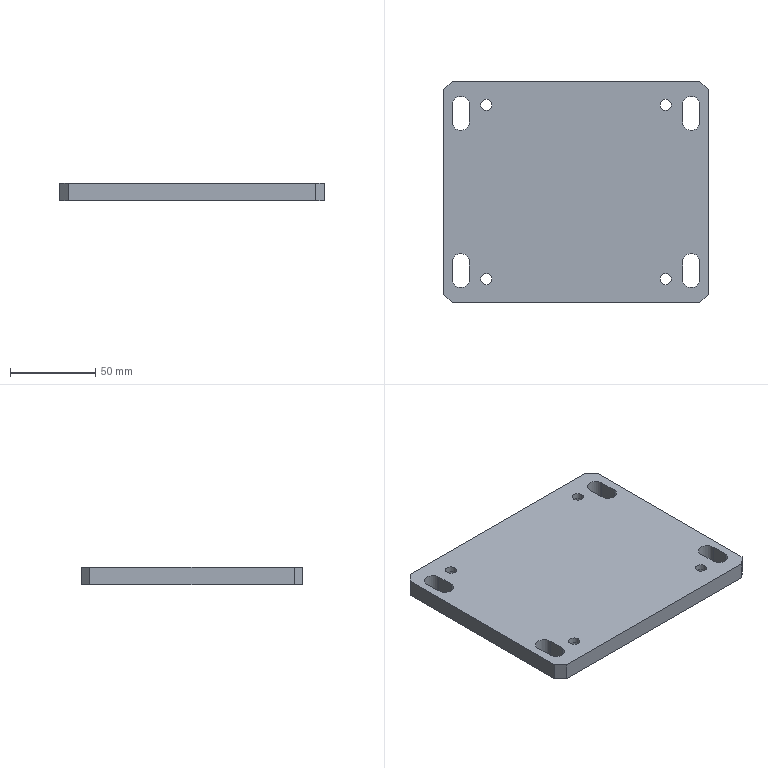CAM job | NX | 3-axis milling, drilling | part box 155 x 130 x 10 mm | stock box 155 x 130 x 10 mm
Tools:
number,name,description,diameter,corner_radius,flute_length,length,flutes
6,D6,平底铣刀-粗,6.0,0.0,25.0,75.0,2
9,D10,平底铣刀-粗,10.0,0.0,35.0,75.0,2
7,D6-J,平底铣刀-精,6.0,0.0,25.0,75.0,2
10,D10-J,平底铣刀-精,10.0,0.0,35.0,75.0,2
2,D6倒角刀,倒角刀,6.0,0.0,3.0,25.0,2
1,C6定点钻,倒角刀,6.0,0.0,3.0,3.0,2
17,ZT6.5,钻头,6.5,0.0,35.0,50.0,2
Operations:
program,operation,operation_type,tool,method,geometry_group,spindle_rpm,surface_speed,feed_per_tooth,feed_cut,feed_plunge,cut_length_mm,path_length_mm,cut_time_min,machine_time_min
B,选线往复层切开粗-中_COPY_1,PlanarMilling,D10,分层开粗-切深K-步距G,W-B,3000.0,94.245,0.3333,2000.0,100.0,1805.117,2433.317,0.9026,0.9654
B,铣倒角_2,PlanarMilling,D6倒角刀,METHOD,W-B,4000.0,75.398,0.075,600.0,100.0,76.787,554.602,0.128,0.1758
B,平面去毛刺6X45L_COPY_1,SurfaceContour,D6倒角刀,爬面_倒角-切深0-步距G,W-B,3500.0,65.972,0.1429,1000.0,100.0,835.116,1413.241,0.8351,0.8929
B,平面铣精光侧面-中-直线_COPY_1,PlanarMilling,D10-J,侧刃精光-切深K-步距G,W-B,3000.0,94.245,0.1333,800.0,100.0,84.284,661.042,0.1054,0.163
A,选线往复层切开粗-中_COPY,PlanarMilling,D10,分层开粗-切深K-步距G,W-A,3000.0,94.245,0.3333,2000.0,100.0,1805.117,2433.317,0.9026,0.9654
A,沉头孔打点-深0.8,Operation,C6定点钻,NONE,W-A,3000.0,56.0,0.01,60.0,90.0,7.2,366.415,0.12,0.1559
A,沉头孔-钻孔0段,Operation,ZT6.5,NONE,W-A,600.0,12.252,0.1,120.0,90.0,59.811,471.637,0.4984,0.5396
A,底壁铣螺旋开粗-中_COPY,VolumeBased25DMillingOperation,D6,分层开粗-切深K-步距G,W-A,4000.0,75.398,0.1875,1500.0,100.0,6790.616,7281.154,4.527,4.576
A,铣孔开粗D6_1,CylinderMilling,D6,NONE,W-A,4000.0,75.398,0.25,2000.0,100.0,1100.907,1339.293,0.5505,0.5743
A,铣孔开粗D6_2,CylinderMilling,D6,NONE,W-A,4000.0,75.398,0.25,2000.0,100.0,1100.907,1339.293,0.5505,0.5743
A,铣倒角_1,PlanarMilling,D6倒角刀,NONE,W-A,4000.0,75.398,0.1,800.0,100.0,173.57,633.91,0.217,0.263
A,平面去毛刺6X45L_COPY,SurfaceContour,D6倒角刀,爬面_倒角-切深0-步距G,W-A,3500.0,65.972,0.1429,1000.0,100.0,891.445,1570.371,0.8914,0.9593
A,铣孔精光D6_1,CylinderMilling,D6-J,精光步距切深关,W-A,4000.0,75.398,0.1,800.0,100.0,89.89,329.276,0.1124,0.1363
A,铣孔精光D6_2,CylinderMilling,D6-J,精光步距切深关,W-A,4000.0,75.398,0.1,800.0,100.0,89.89,329.276,0.1124,0.1363
A,底壁铣螺旋精光-中_COPY,VolumeBased25DMillingOperation,D6-J,螺旋精光-切深K-步距G,W-A,3500.0,65.972,0.1143,800.0,100.0,567.715,1087.639,0.7096,0.7616
A,平面铣精光侧面-中-直线_COPY,PlanarMilling,D10-J,侧刃精光-切深K-步距G,W-A,3000.0,94.245,0.1333,800.0,100.0,84.284,661.042,0.1054,0.163